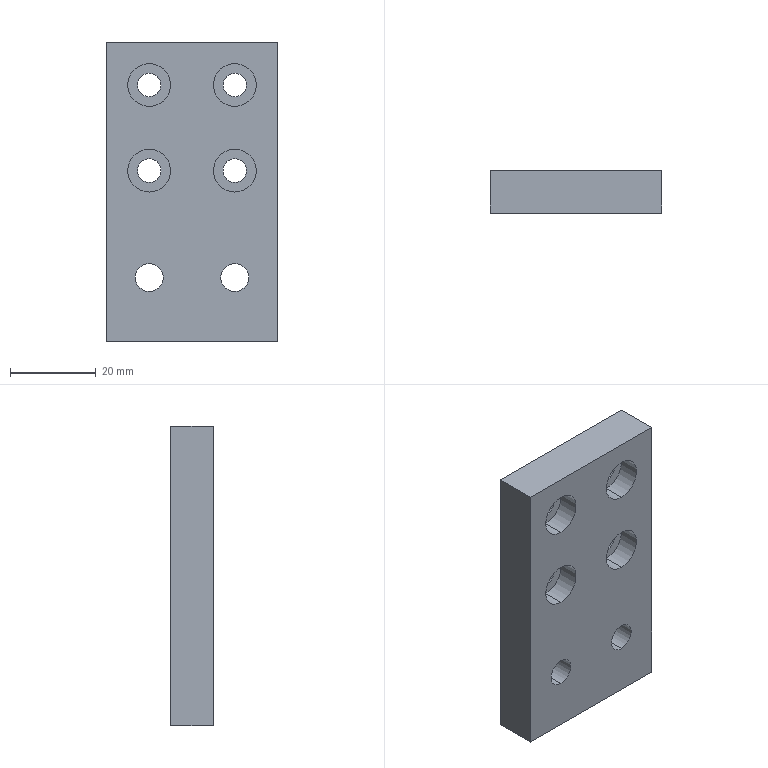Part | STEP file | 0245_211_Plate | 1 solid | 30 faces | box 40 x 10 x 70 mm | volume 25290 mm3 | cylinder 20 | plane 10 | commonest cylinder face diameters 5.5 x8 10 x8 6.5 x4